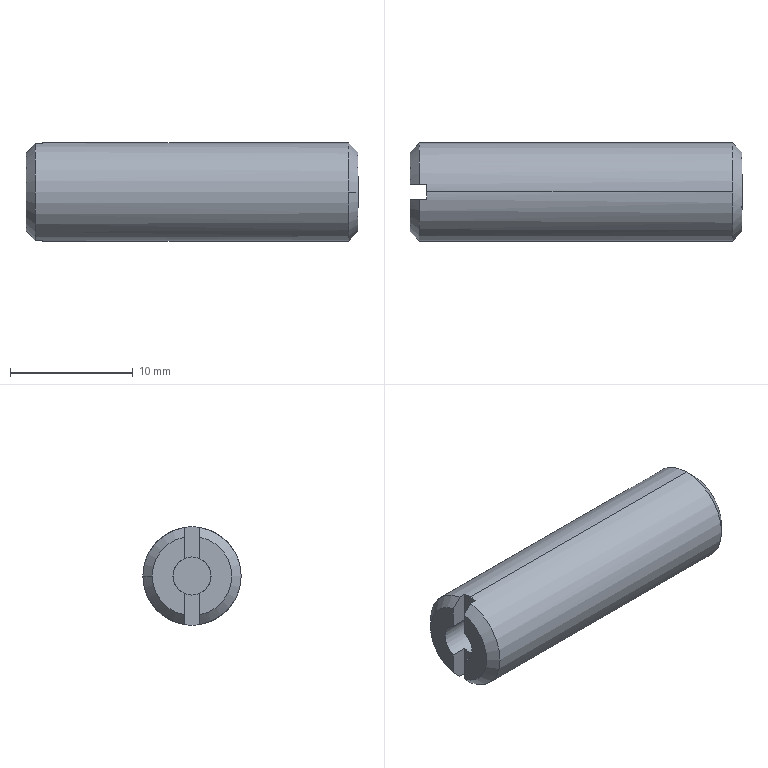Part | SolidWorks | features BaseBody 1 | 1 solid | 29 faces | box 27 x 8 x 8 mm | volume 931.32 mm3 | plane 18 | cylinder 6 | cone 5 | commonest cylinder face diameters 3.1 x2 4.8 x2 8 x2
STEP:
#1=CARTESIAN_POINT('',(26.233,4.,0.));
#2=VERTEX_POINT('',#1);
#3=CARTESIAN_POINT('',(26.233,0.,-4.));
#4=VERTEX_POINT('',#3);
#5=CARTESIAN_POINT('',(26.233,0.,0.));
#6=DIRECTION('',(-1.,0.,0.));
#7=DIRECTION('',(0.,0.,1.));
#8=AXIS2_PLACEMENT_3D('',#5,#6,#7);
#9=CIRCLE('',#8,4.);
#10=EDGE_CURVE('',#2,#4,#9,.T.);
#11=ORIENTED_EDGE('',*,*,#10,.T.);
#12=CARTESIAN_POINT('',(1.35,0.,-4.));
#13=VERTEX_POINT('',#12);
#14=CARTESIAN_POINT('',(27.,0.,-4.));
#15=DIRECTION('',(-1.,0.,0.));
#16=VECTOR('',#15,1000.);
#17=LINE('',#14,#16);
#18=EDGE_CURVE('',#4,#13,#17,.T.);
#19=ORIENTED_EDGE('',*,*,#18,.T.);
#20=CARTESIAN_POINT('',(1.35,0.62,-3.952));
#21=VERTEX_POINT('',#20);
#22=CARTESIAN_POINT('',(1.35,0.,0.));
#23=DIRECTION('',(1.,0.,0.));
#24=DIRECTION('',(0.,0.,1.));
#25=AXIS2_PLACEMENT_3D('',#22,#23,#24);
#26=CIRCLE('',#25,4.);
#27=EDGE_CURVE('',#13,#21,#26,.T.);
#28=ORIENTED_EDGE('',*,*,#27,.T.);
#29=CARTESIAN_POINT('',(0.767,0.62,-3.952));
#30=VERTEX_POINT('',#29);
#31=CARTESIAN_POINT('',(1.35,0.62,-3.952));
#32=DIRECTION('',(1.,0.,0.));
#33=VECTOR('',#32,1000.);
#34=LINE('',#31,#33);
#35=EDGE_CURVE('',#30,#21,#34,.T.);
#36=ORIENTED_EDGE('',*,*,#35,.F.);
#37=CARTESIAN_POINT('',(0.767,4.,0.));
#38=VERTEX_POINT('',#37);
#39=CARTESIAN_POINT('',(0.767,0.,0.));
#40=DIRECTION('',(1.,0.,0.));
#41=DIRECTION('',(0.,0.,1.));
#42=AXIS2_PLACEMENT_3D('',#39,#40,#41);
#43=CIRCLE('',#42,4.);
#44=EDGE_CURVE('',#30,#38,#43,.T.);
#45=ORIENTED_EDGE('',*,*,#44,.T.);
#46=CARTESIAN_POINT('',(0.767,0.62,3.952));
#47=VERTEX_POINT('',#46);
#48=CARTESIAN_POINT('',(0.767,0.,0.));
#49=DIRECTION('',(1.,0.,0.));
#50=DIRECTION('',(0.,0.,1.));
#51=AXIS2_PLACEMENT_3D('',#48,#49,#50);
#52=CIRCLE('',#51,4.);
#53=EDGE_CURVE('',#38,#47,#52,.T.);
#54=ORIENTED_EDGE('',*,*,#53,.T.);
#55=CARTESIAN_POINT('',(1.35,0.62,3.952));
#56=VERTEX_POINT('',#55);
#57=CARTESIAN_POINT('',(1.35,0.62,3.952));
#58=DIRECTION('',(-1.,0.,0.));
#59=VECTOR('',#58,1000.);
#60=LINE('',#57,#59);
#61=EDGE_CURVE('',#56,#47,#60,.T.);
#62=ORIENTED_EDGE('',*,*,#61,.F.);
#63=CARTESIAN_POINT('',(1.35,0.,4.));
#64=VERTEX_POINT('',#63);
#65=CARTESIAN_POINT('',(1.35,0.,0.));
#66=DIRECTION('',(1.,0.,0.));
#67=DIRECTION('',(0.,0.,1.));
#68=AXIS2_PLACEMENT_3D('',#65,#66,#67);
#69=CIRCLE('',#68,4.);
#70=EDGE_CURVE('',#56,#64,#69,.T.);
#71=ORIENTED_EDGE('',*,*,#70,.T.);
#72=CARTESIAN_POINT('',(26.233,0.,4.));
#73=VERTEX_POINT('',#72);
#74=CARTESIAN_POINT('',(27.,0.,4.));
#75=DIRECTION('',(-1.,0.,0.));
#76=VECTOR('',#75,1000.);
#77=LINE('',#74,#76);
#78=EDGE_CURVE('',#73,#64,#77,.T.);
#79=ORIENTED_EDGE('',*,*,#78,.F.);
#80=CARTESIAN_POINT('',(26.233,0.,0.));
#81=DIRECTION('',(-1.,0.,0.));
#82=DIRECTION('',(0.,0.,1.));
#83=AXIS2_PLACEMENT_3D('',#80,#81,#82);
#84=CIRCLE('',#83,4.);
#85=EDGE_CURVE('',#73,#2,#84,.T.);
#86=ORIENTED_EDGE('',*,*,#85,.T.);
#87=EDGE_LOOP('',(#11,#19,#28,#36,#45,#54,#62,#71,#79,#86));
#88=FACE_OUTER_BOUND('',#87,.T.);
#89=CARTESIAN_POINT('',(27.,0.,0.));
#90=DIRECTION('',(-1.,0.,0.));
#91=DIRECTION('',(0.,0.,1.));
#92=AXIS2_PLACEMENT_3D('',#89,#90,#91);
#93=CYLINDRICAL_SURFACE('',#92,4.);
#94=ADVANCED_FACE('',(#88),#93,.T.);
#95=CARTESIAN_POINT('',(27.,-3.233,0.));
#96=VERTEX_POINT('',#95);
#97=CARTESIAN_POINT('',(27.,3.233,0.));
#98=VERTEX_POINT('',#97);
#99=CARTESIAN_POINT('',(27.,0.,0.));
#100=DIRECTION('',(-1.,0.,0.));
#101=DIRECTION('',(0.,-1.,0.));
#102=AXIS2_PLACEMENT_3D('',#99,#100,#101);
#103=CIRCLE('',#102,3.233);
#104=EDGE_CURVE('',#96,#98,#103,.T.);
#105=ORIENTED_EDGE('',*,*,#104,.T.);
#106=CARTESIAN_POINT('',(26.233,4.,0.));
#107=DIRECTION('',(-0.7071,0.7071,0.));
#108=VECTOR('',#107,1000.);
#109=LINE('',#106,#108);
#110=EDGE_CURVE('',#98,#2,#109,.T.);
#111=ORIENTED_EDGE('',*,*,#110,.T.);
#112=ORIENTED_EDGE('',*,*,#85,.F.);
#113=CARTESIAN_POINT('',(26.233,-4.,0.));
#114=VERTEX_POINT('',#113);
#115=CARTESIAN_POINT('',(26.233,0.,0.));
#116=DIRECTION('',(-1.,0.,0.));
#117=DIRECTION('',(0.,0.,1.));
#118=AXIS2_PLACEMENT_3D('',#115,#116,#117);
#119=CIRCLE('',#118,4.);
#120=EDGE_CURVE('',#114,#73,#119,.T.);
#121=ORIENTED_EDGE('',*,*,#120,.F.);
#122=CARTESIAN_POINT('',(26.233,-4.,0.));
#123=DIRECTION('',(-0.7071,-0.7071,0.));
#124=VECTOR('',#123,1000.);
#125=LINE('',#122,#124);
#126=EDGE_CURVE('',#96,#114,#125,.T.);
#127=ORIENTED_EDGE('',*,*,#126,.F.);
#128=EDGE_LOOP('',(#105,#111,#112,#121,#127));
#129=FACE_OUTER_BOUND('',#128,.T.);
#130=CARTESIAN_POINT('',(26.233,0.,0.));
#131=DIRECTION('',(-1.,0.,0.));
#132=DIRECTION('',(0.,-1.,0.));
#133=AXIS2_PLACEMENT_3D('',#130,#131,#132);
#134=CONICAL_SURFACE('',#133,4.,0.7854);
#135=ADVANCED_FACE('',(#129),#134,.T.);
#136=CARTESIAN_POINT('',(0.,0.62,-3.173));
#137=VERTEX_POINT('',#136);
#138=CARTESIAN_POINT('',(0.,3.233,0.));
#139=VERTEX_POINT('',#138);
#140=CARTESIAN_POINT('',(0.,0.,0.));
#141=DIRECTION('',(1.,0.,0.));
#142=DIRECTION('',(0.,1.,0.));
#143=AXIS2_PLACEMENT_3D('',#140,#141,#142);
#144=CIRCLE('',#143,3.233);
#145=EDGE_CURVE('',#137,#139,#144,.T.);
#146=ORIENTED_EDGE('',*,*,#145,.T.);
#147=CARTESIAN_POINT('',(0.767,4.,0.));
#148=DIRECTION('',(0.7071,0.7071,0.));
#149=VECTOR('',#148,1000.);
#150=LINE('',#147,#149);
#151=EDGE_CURVE('',#139,#38,#150,.T.);
#152=ORIENTED_EDGE('',*,*,#151,.T.);
#153=ORIENTED_EDGE('',*,*,#44,.F.);
#154=CARTESIAN_POINT('',(0.,0.62,-3.173));
#155=CARTESIAN_POINT('',(0.2552,0.62,-3.433));
#156=CARTESIAN_POINT('',(0.511,0.62,-3.692));
#157=CARTESIAN_POINT('',(0.767,0.62,-3.952));
#158=B_SPLINE_CURVE_WITH_KNOTS('',3,(#154,#155,#156,#157),.UNSPECIFIED.,.F.,.F.,(4,4),(0.,0.001093),.UNSPECIFIED.);
#159=EDGE_CURVE('',#137,#30,#158,.T.);
#160=ORIENTED_EDGE('',*,*,#159,.F.);
#161=EDGE_LOOP('',(#146,#152,#153,#160));
#162=FACE_OUTER_BOUND('',#161,.T.);
#163=CARTESIAN_POINT('',(0.767,0.,0.));
#164=DIRECTION('',(1.,0.,0.));
#165=DIRECTION('',(0.,1.,0.));
#166=AXIS2_PLACEMENT_3D('',#163,#164,#165);
#167=CONICAL_SURFACE('',#166,4.,0.7854);
#168=ADVANCED_FACE('',(#162),#167,.T.);
#169=CARTESIAN_POINT('',(4.5,0.,-1.55));
#170=VERTEX_POINT('',#169);
#171=CARTESIAN_POINT('',(4.5,0.,1.55));
#172=VERTEX_POINT('',#171);
#173=CARTESIAN_POINT('',(4.5,0.,0.));
#174=DIRECTION('',(-1.,0.,0.));
#175=DIRECTION('',(0.,0.,1.));
#176=AXIS2_PLACEMENT_3D('',#173,#174,#175);
#177=CIRCLE('',#176,1.55);
#178=EDGE_CURVE('',#170,#172,#177,.T.);
#179=ORIENTED_EDGE('',*,*,#178,.F.);
#180=CARTESIAN_POINT('',(1.35,0.,-1.55));
#181=VERTEX_POINT('',#180);
#182=CARTESIAN_POINT('',(27.,0.,-1.55));
#183=DIRECTION('',(-1.,0.,0.));
#184=VECTOR('',#183,1000.);
#185=LINE('',#182,#184);
#186=EDGE_CURVE('',#170,#181,#185,.T.);
#187=ORIENTED_EDGE('',*,*,#186,.T.);
#188=CARTESIAN_POINT('',(1.35,-0.62,-1.421));
#189=VERTEX_POINT('',#188);
#190=CARTESIAN_POINT('',(1.35,0.,0.));
#191=DIRECTION('',(1.,0.,0.));
#192=DIRECTION('',(0.,0.,1.));
#193=AXIS2_PLACEMENT_3D('',#190,#191,#192);
#194=CIRCLE('',#193,1.55);
#195=EDGE_CURVE('',#189,#181,#194,.T.);
#196=ORIENTED_EDGE('',*,*,#195,.F.);
#197=CARTESIAN_POINT('',(0.,-0.62,-1.421));
#198=VERTEX_POINT('',#197);
#199=CARTESIAN_POINT('',(27.,-0.62,-1.421));
#200=DIRECTION('',(1.,0.,0.));
#201=VECTOR('',#200,1000.);
#202=LINE('',#199,#201);
#203=EDGE_CURVE('',#198,#189,#202,.T.);
#204=ORIENTED_EDGE('',*,*,#203,.F.);
#205=CARTESIAN_POINT('',(0.,-0.62,1.421));
#206=VERTEX_POINT('',#205);
#207=CARTESIAN_POINT('',(0.,0.,0.));
#208=DIRECTION('',(-1.,0.,0.));
#209=DIRECTION('',(0.,0.,1.));
#210=AXIS2_PLACEMENT_3D('',#207,#208,#209);
#211=CIRCLE('',#210,1.55);
#212=EDGE_CURVE('',#198,#206,#211,.T.);
#213=ORIENTED_EDGE('',*,*,#212,.T.);
#214=CARTESIAN_POINT('',(1.35,-0.62,1.421));
#215=VERTEX_POINT('',#214);
#216=CARTESIAN_POINT('',(1.35,-0.62,1.421));
#217=DIRECTION('',(-1.,0.,0.));
#218=VECTOR('',#217,1000.);
#219=LINE('',#216,#218);
#220=EDGE_CURVE('',#215,#206,#219,.T.);
#221=ORIENTED_EDGE('',*,*,#220,.F.);
#222=CARTESIAN_POINT('',(1.35,0.,1.55));
#223=VERTEX_POINT('',#222);
#224=CARTESIAN_POINT('',(1.35,0.,0.));
#225=DIRECTION('',(1.,0.,0.));
#226=DIRECTION('',(0.,0.,1.));
#227=AXIS2_PLACEMENT_3D('',#224,#225,#226);
#228=CIRCLE('',#227,1.55);
#229=EDGE_CURVE('',#223,#215,#228,.T.);
#230=ORIENTED_EDGE('',*,*,#229,.F.);
#231=CARTESIAN_POINT('',(27.,0.,1.55));
#232=DIRECTION('',(-1.,0.,0.));
#233=VECTOR('',#232,1000.);
#234=LINE('',#231,#233);
#235=EDGE_CURVE('',#172,#223,#234,.T.);
#236=ORIENTED_EDGE('',*,*,#235,.F.);
#237=EDGE_LOOP('',(#179,#187,#196,#204,#213,#221,#230,#236));
#238=FACE_OUTER_BOUND('',#237,.T.);
#239=CARTESIAN_POINT('',(27.,0.,0.));
#240=DIRECTION('',(-1.,0.,0.));
#241=DIRECTION('',(0.,0.,1.));
#242=AXIS2_PLACEMENT_3D('',#239,#240,#241);
#243=CYLINDRICAL_SURFACE('',#242,1.55);
#244=ADVANCED_FACE('',(#238),#243,.F.);
#245=CARTESIAN_POINT('',(24.57,0.,-2.4));
#246=VERTEX_POINT('',#245);
#247=CARTESIAN_POINT('',(24.57,0.,2.4));
#248=VERTEX_POINT('',#247);
#249=CARTESIAN_POINT('',(24.57,0.,0.));
#250=DIRECTION('',(-1.,0.,0.));
#251=DIRECTION('',(0.,0.,1.));
#252=AXIS2_PLACEMENT_3D('',#249,#250,#251);
#253=CIRCLE('',#252,2.4);
#254=EDGE_CURVE('',#246,#248,#253,.T.);
#255=ORIENTED_EDGE('',*,*,#254,.F.);
#256=CARTESIAN_POINT('',(4.5,0.,-2.4));
#257=VERTEX_POINT('',#256);
#258=CARTESIAN_POINT('',(27.,0.,-2.4));
#259=DIRECTION('',(-1.,0.,0.));
#260=VECTOR('',#259,1000.);
#261=LINE('',#258,#260);
#262=EDGE_CURVE('',#246,#257,#261,.T.);
#263=ORIENTED_EDGE('',*,*,#262,.T.);
#264=CARTESIAN_POINT('',(4.5,0.,2.4));
#265=VERTEX_POINT('',#264);
#266=CARTESIAN_POINT('',(4.5,0.,0.));
#267=DIRECTION('',(-1.,0.,0.));
#268=DIRECTION('',(0.,0.,1.));
#269=AXIS2_PLACEMENT_3D('',#266,#267,#268);
#270=CIRCLE('',#269,2.4);
#271=EDGE_CURVE('',#257,#265,#270,.T.);
#272=ORIENTED_EDGE('',*,*,#271,.T.);
#273=CARTESIAN_POINT('',(27.,0.,2.4));
#274=DIRECTION('',(-1.,0.,0.));
#275=VECTOR('',#274,1000.);
#276=LINE('',#273,#275);
#277=EDGE_CURVE('',#248,#265,#276,.T.);
#278=ORIENTED_EDGE('',*,*,#277,.F.);
#279=EDGE_LOOP('',(#255,#263,#272,#278));
#280=FACE_OUTER_BOUND('',#279,.T.);
#281=CARTESIAN_POINT('',(27.,0.,0.));
#282=DIRECTION('',(-1.,0.,0.));
#283=DIRECTION('',(0.,0.,1.));
#284=AXIS2_PLACEMENT_3D('',#281,#282,#283);
#285=CYLINDRICAL_SURFACE('',#284,2.4);
#286=ADVANCED_FACE('',(#280),#285,.F.);
#287=ORIENTED_EDGE('',*,*,#18,.F.);
#288=CARTESIAN_POINT('',(26.233,0.,0.));
#289=DIRECTION('',(-1.,0.,0.));
#290=DIRECTION('',(0.,0.,1.));
#291=AXIS2_PLACEMENT_3D('',#288,#289,#290);
#292=CIRCLE('',#291,4.);
#293=EDGE_CURVE('',#4,#114,#292,.T.);
#294=ORIENTED_EDGE('',*,*,#293,.T.);
#295=ORIENTED_EDGE('',*,*,#120,.T.);
#296=ORIENTED_EDGE('',*,*,#78,.T.);
#297=CARTESIAN_POINT('',(1.35,-0.62,3.952));
#298=VERTEX_POINT('',#297);
#299=CARTESIAN_POINT('',(1.35,0.,0.));
#300=DIRECTION('',(1.,0.,0.));
#301=DIRECTION('',(0.,0.,1.));
#302=AXIS2_PLACEMENT_3D('',#299,#300,#301);
#303=CIRCLE('',#302,4.);
#304=EDGE_CURVE('',#64,#298,#303,.T.);
#305=ORIENTED_EDGE('',*,*,#304,.T.);
#306=CARTESIAN_POINT('',(0.767,-0.62,3.952));
#307=VERTEX_POINT('',#306);
#308=CARTESIAN_POINT('',(1.35,-0.62,3.952));
#309=DIRECTION('',(1.,0.,0.));
#310=VECTOR('',#309,1000.);
#311=LINE('',#308,#310);
#312=EDGE_CURVE('',#307,#298,#311,.T.);
#313=ORIENTED_EDGE('',*,*,#312,.F.);
#314=CARTESIAN_POINT('',(0.767,-0.62,-3.952));
#315=VERTEX_POINT('',#314);
#316=CARTESIAN_POINT('',(0.767,0.,0.));
#317=DIRECTION('',(1.,0.,0.));
#318=DIRECTION('',(0.,0.,1.));
#319=AXIS2_PLACEMENT_3D('',#316,#317,#318);
#320=CIRCLE('',#319,4.);
#321=EDGE_CURVE('',#307,#315,#320,.T.);
#322=ORIENTED_EDGE('',*,*,#321,.T.);
#323=CARTESIAN_POINT('',(1.35,-0.62,-3.952));
#324=VERTEX_POINT('',#323);
#325=CARTESIAN_POINT('',(1.35,-0.62,-3.952));
#326=DIRECTION('',(-1.,0.,0.));
#327=VECTOR('',#326,1000.);
#328=LINE('',#325,#327);
#329=EDGE_CURVE('',#324,#315,#328,.T.);
#330=ORIENTED_EDGE('',*,*,#329,.F.);
#331=CARTESIAN_POINT('',(1.35,0.,0.));
#332=DIRECTION('',(1.,0.,0.));
#333=DIRECTION('',(0.,0.,1.));
#334=AXIS2_PLACEMENT_3D('',#331,#332,#333);
#335=CIRCLE('',#334,4.);
#336=EDGE_CURVE('',#324,#13,#335,.T.);
#337=ORIENTED_EDGE('',*,*,#336,.T.);
#338=EDGE_LOOP('',(#287,#294,#295,#296,#305,#313,#322,#330,#337));
#339=FACE_OUTER_BOUND('',#338,.T.);
#340=CARTESIAN_POINT('',(27.,0.,0.));
#341=DIRECTION('',(-1.,0.,0.));
#342=DIRECTION('',(0.,0.,1.));
#343=AXIS2_PLACEMENT_3D('',#340,#341,#342);
#344=CYLINDRICAL_SURFACE('',#343,4.);
#345=ADVANCED_FACE('',(#339),#344,.T.);
#346=CARTESIAN_POINT('',(0.,-0.62,-3.173));
#347=VERTEX_POINT('',#346);
#348=CARTESIAN_POINT('',(0.767,-0.62,-3.952));
#349=CARTESIAN_POINT('',(0.511,-0.62,-3.692));
#350=CARTESIAN_POINT('',(0.2552,-0.62,-3.433));
#351=CARTESIAN_POINT('',(0.,-0.62,-3.173));
#352=B_SPLINE_CURVE_WITH_KNOTS('',3,(#348,#349,#350,#351),.UNSPECIFIED.,.F.,.F.,(4,4),(0.,0.001093),.UNSPECIFIED.);
#353=EDGE_CURVE('',#315,#347,#352,.T.);
#354=ORIENTED_EDGE('',*,*,#353,.F.);
#355=ORIENTED_EDGE('',*,*,#321,.F.);
#356=CARTESIAN_POINT('',(0.,-0.62,3.173));
#357=VERTEX_POINT('',#356);
#358=CARTESIAN_POINT('',(0.,-0.62,3.173));
#359=CARTESIAN_POINT('',(0.2552,-0.62,3.433));
#360=CARTESIAN_POINT('',(0.511,-0.62,3.692));
#361=CARTESIAN_POINT('',(0.767,-0.62,3.952));
#362=B_SPLINE_CURVE_WITH_KNOTS('',3,(#358,#359,#360,#361),.UNSPECIFIED.,.F.,.F.,(4,4),(0.,0.001093),.UNSPECIFIED.);
#363=EDGE_CURVE('',#357,#307,#362,.T.);
#364=ORIENTED_EDGE('',*,*,#363,.F.);
#365=CARTESIAN_POINT('',(0.,0.,0.));
#366=DIRECTION('',(1.,0.,0.));
#367=DIRECTION('',(0.,1.,0.));
#368=AXIS2_PLACEMENT_3D('',#365,#366,#367);
#369=CIRCLE('',#368,3.233);
#370=EDGE_CURVE('',#357,#347,#369,.T.);
#371=ORIENTED_EDGE('',*,*,#370,.T.);
#372=EDGE_LOOP('',(#354,#355,#364,#371));
#373=FACE_OUTER_BOUND('',#372,.T.);
#374=CARTESIAN_POINT('',(0.767,0.,0.));
#375=DIRECTION('',(1.,0.,0.));
#376=DIRECTION('',(0.,1.,0.));
#377=AXIS2_PLACEMENT_3D('',#374,#375,#376);
#378=CONICAL_SURFACE('',#377,4.,0.7854);
#379=ADVANCED_FACE('',(#373),#378,.T.);
#380=ORIENTED_EDGE('',*,*,#110,.F.);
#381=CARTESIAN_POINT('',(27.,0.,0.));
#382=DIRECTION('',(-1.,0.,0.));
#383=DIRECTION('',(0.,-1.,0.));
#384=AXIS2_PLACEMENT_3D('',#381,#382,#383);
#385=CIRCLE('',#384,3.233);
#386=EDGE_CURVE('',#98,#96,#385,.T.);
#387=ORIENTED_EDGE('',*,*,#386,.T.);
#388=ORIENTED_EDGE('',*,*,#126,.T.);
#389=ORIENTED_EDGE('',*,*,#293,.F.);
#390=ORIENTED_EDGE('',*,*,#10,.F.);
#391=EDGE_LOOP('',(#380,#387,#388,#389,#390));
#392=FACE_OUTER_BOUND('',#391,.T.);
#393=CARTESIAN_POINT('',(26.233,0.,0.));
#394=DIRECTION('',(-1.,0.,0.));
#395=DIRECTION('',(0.,-1.,0.));
#396=AXIS2_PLACEMENT_3D('',#393,#394,#395);
#397=CONICAL_SURFACE('',#396,4.,0.7854);
#398=ADVANCED_FACE('',(#392),#397,.T.);
#399=CARTESIAN_POINT('',(0.,-0.62,0.));
#400=DIRECTION('',(0.,0.,1.));
#401=VECTOR('',#400,1000.);
#402=LINE('',#399,#401);
#403=EDGE_CURVE('',#206,#357,#402,.T.);
#404=ORIENTED_EDGE('',*,*,#403,.F.);
#405=ORIENTED_EDGE('',*,*,#212,.F.);
#406=CARTESIAN_POINT('',(0.,-0.62,0.));
#407=DIRECTION('',(0.,0.,1.));
#408=VECTOR('',#407,1000.);
#409=LINE('',#406,#408);
#410=EDGE_CURVE('',#347,#198,#409,.T.);
#411=ORIENTED_EDGE('',*,*,#410,.F.);
#412=ORIENTED_EDGE('',*,*,#370,.F.);
#413=EDGE_LOOP('',(#404,#405,#411,#412));
#414=FACE_OUTER_BOUND('',#413,.T.);
#415=CARTESIAN_POINT('',(0.,1.55,0.));
#416=DIRECTION('',(1.,0.,0.));
#417=DIRECTION('',(0.,0.,-1.));
#418=AXIS2_PLACEMENT_3D('',#415,#416,#417);
#419=PLANE('',#418);
#420=ADVANCED_FACE('',(#414),#419,.F.);
#421=ORIENTED_EDGE('',*,*,#151,.F.);
#422=CARTESIAN_POINT('',(0.,0.62,3.173));
#423=VERTEX_POINT('',#422);
#424=CARTESIAN_POINT('',(0.,0.,0.));
#425=DIRECTION('',(1.,0.,0.));
#426=DIRECTION('',(0.,1.,0.));
#427=AXIS2_PLACEMENT_3D('',#424,#425,#426);
#428=CIRCLE('',#427,3.233);
#429=EDGE_CURVE('',#139,#423,#428,.T.);
#430=ORIENTED_EDGE('',*,*,#429,.T.);
#431=CARTESIAN_POINT('',(0.767,0.62,3.952));
#432=CARTESIAN_POINT('',(0.511,0.62,3.692));
#433=CARTESIAN_POINT('',(0.2552,0.62,3.433));
#434=CARTESIAN_POINT('',(0.,0.62,3.173));
#435=B_SPLINE_CURVE_WITH_KNOTS('',3,(#431,#432,#433,#434),.UNSPECIFIED.,.F.,.F.,(4,4),(0.,0.001093),.UNSPECIFIED.);
#436=EDGE_CURVE('',#47,#423,#435,.T.);
#437=ORIENTED_EDGE('',*,*,#436,.F.);
#438=ORIENTED_EDGE('',*,*,#53,.F.);
#439=EDGE_LOOP('',(#421,#430,#437,#438));
#440=FACE_OUTER_BOUND('',#439,.T.);
#441=CARTESIAN_POINT('',(0.767,0.,0.));
#442=DIRECTION('',(1.,0.,0.));
#443=DIRECTION('',(0.,1.,0.));
#444=AXIS2_PLACEMENT_3D('',#441,#442,#443);
#445=CONICAL_SURFACE('',#444,4.,0.7854);
#446=ADVANCED_FACE('',(#440),#445,.T.);
#447=CARTESIAN_POINT('',(27.,-0.7217,-1.25));
#448=VERTEX_POINT('',#447);
#449=CARTESIAN_POINT('',(27.,0.7217,-1.25));
#450=VERTEX_POINT('',#449);
#451=CARTESIAN_POINT('',(27.,3.233,-1.25));
#452=DIRECTION('',(0.,1.,0.));
#453=VECTOR('',#452,1000.);
#454=LINE('',#451,#453);
#455=EDGE_CURVE('',#448,#450,#454,.T.);
#456=ORIENTED_EDGE('',*,*,#455,.F.);
#457=CARTESIAN_POINT('',(27.,-1.443,0.));
#458=VERTEX_POINT('',#457);
#459=CARTESIAN_POINT('',(27.,-1.443,0.));
#460=DIRECTION('',(0.,0.5,-0.866));
#461=VECTOR('',#460,1000.);
#462=LINE('',#459,#461);
#463=EDGE_CURVE('',#458,#448,#462,.T.);
#464=ORIENTED_EDGE('',*,*,#463,.F.);
#465=CARTESIAN_POINT('',(27.,-0.7217,1.25));
#466=VERTEX_POINT('',#465);
#467=CARTESIAN_POINT('',(27.,-0.7217,1.25));
#468=DIRECTION('',(0.,-0.5,-0.866));
#469=VECTOR('',#468,1000.);
#470=LINE('',#467,#469);
#471=EDGE_CURVE('',#466,#458,#470,.T.);
#472=ORIENTED_EDGE('',*,*,#471,.F.);
#473=CARTESIAN_POINT('',(27.,0.7217,1.25));
#474=VERTEX_POINT('',#473);
#475=CARTESIAN_POINT('',(27.,3.233,1.25));
#476=DIRECTION('',(0.,-1.,0.));
#477=VECTOR('',#476,1000.);
#478=LINE('',#475,#477);
#479=EDGE_CURVE('',#474,#466,#478,.T.);
#480=ORIENTED_EDGE('',*,*,#479,.F.);
#481=CARTESIAN_POINT('',(27.,1.443,0.));
#482=VERTEX_POINT('',#481);
#483=CARTESIAN_POINT('',(27.,1.443,0.));
#484=DIRECTION('',(0.,-0.5,0.866));
#485=VECTOR('',#484,1000.);
#486=LINE('',#483,#485);
#487=EDGE_CURVE('',#482,#474,#486,.T.);
#488=ORIENTED_EDGE('',*,*,#487,.F.);
#489=CARTESIAN_POINT('',(27.,0.7217,-1.25));
#490=DIRECTION('',(0.,0.5,0.866));
#491=VECTOR('',#490,1000.);
#492=LINE('',#489,#491);
#493=EDGE_CURVE('',#450,#482,#492,.T.);
#494=ORIENTED_EDGE('',*,*,#493,.F.);
#495=EDGE_LOOP('',(#456,#464,#472,#480,#488,#494));
#496=FACE_BOUND('',#495,.T.);
#497=ORIENTED_EDGE('',*,*,#104,.F.);
#498=ORIENTED_EDGE('',*,*,#386,.F.);
#499=EDGE_LOOP('',(#497,#498));
#500=FACE_OUTER_BOUND('',#499,.T.);
#501=CARTESIAN_POINT('',(27.,3.233,0.));
#502=DIRECTION('',(-1.,0.,0.));
#503=DIRECTION('',(0.,0.,1.));
#504=AXIS2_PLACEMENT_3D('',#501,#502,#503);
#505=PLANE('',#504);
#506=ADVANCED_FACE('',(#496,#500),#505,.F.);
#507=ORIENTED_EDGE('',*,*,#403,.T.);
#508=ORIENTED_EDGE('',*,*,#363,.T.);
#509=ORIENTED_EDGE('',*,*,#312,.T.);
#510=CARTESIAN_POINT('',(1.35,-0.62,8.));
#511=DIRECTION('',(0.,0.,-1.));
#512=VECTOR('',#511,1000.);
#513=LINE('',#510,#512);
#514=EDGE_CURVE('',#298,#215,#513,.T.);
#515=ORIENTED_EDGE('',*,*,#514,.T.);
#516=ORIENTED_EDGE('',*,*,#220,.T.);
#517=EDGE_LOOP('',(#507,#508,#509,#515,#516));
#518=FACE_OUTER_BOUND('',#517,.T.);
#519=CARTESIAN_POINT('',(1.35,-0.62,8.));
#520=DIRECTION('',(0.,1.,0.));
#521=DIRECTION('',(0.,0.,1.));
#522=AXIS2_PLACEMENT_3D('',#519,#520,#521);
#523=PLANE('',#522);
#524=ADVANCED_FACE('',(#518),#523,.T.);
#525=ORIENTED_EDGE('',*,*,#186,.F.);
#526=CARTESIAN_POINT('',(4.5,0.,0.));
#527=DIRECTION('',(-1.,0.,0.));
#528=DIRECTION('',(0.,0.,1.));
#529=AXIS2_PLACEMENT_3D('',#526,#527,#528);
#530=CIRCLE('',#529,1.55);
#531=EDGE_CURVE('',#172,#170,#530,.T.);
#532=ORIENTED_EDGE('',*,*,#531,.F.);
#533=ORIENTED_EDGE('',*,*,#235,.T.);
#534=CARTESIAN_POINT('',(1.35,0.62,1.421));
#535=VERTEX_POINT('',#534);
#536=CARTESIAN_POINT('',(1.35,0.,0.));
#537=DIRECTION('',(1.,0.,0.));
#538=DIRECTION('',(0.,0.,1.));
#539=AXIS2_PLACEMENT_3D('',#536,#537,#538);
#540=CIRCLE('',#539,1.55);
#541=EDGE_CURVE('',#535,#223,#540,.T.);
#542=ORIENTED_EDGE('',*,*,#541,.F.);
#543=CARTESIAN_POINT('',(0.,0.62,1.421));
#544=VERTEX_POINT('',#543);
#545=CARTESIAN_POINT('',(27.,0.62,1.421));
#546=DIRECTION('',(1.,0.,0.));
#547=VECTOR('',#546,1000.);
#548=LINE('',#545,#547);
#549=EDGE_CURVE('',#544,#535,#548,.T.);
#550=ORIENTED_EDGE('',*,*,#549,.F.);
#551=CARTESIAN_POINT('',(0.,0.62,-1.421));
#552=VERTEX_POINT('',#551);
#553=CARTESIAN_POINT('',(0.,0.,0.));
#554=DIRECTION('',(-1.,0.,0.));
#555=DIRECTION('',(0.,0.,1.));
#556=AXIS2_PLACEMENT_3D('',#553,#554,#555);
#557=CIRCLE('',#556,1.55);
#558=EDGE_CURVE('',#544,#552,#557,.T.);
#559=ORIENTED_EDGE('',*,*,#558,.T.);
#560=CARTESIAN_POINT('',(1.35,0.62,-1.421));
#561=VERTEX_POINT('',#560);
#562=CARTESIAN_POINT('',(27.,0.62,-1.421));
#563=DIRECTION('',(-1.,0.,0.));
#564=VECTOR('',#563,1000.);
#565=LINE('',#562,#564);
#566=EDGE_CURVE('',#561,#552,#565,.T.);
#567=ORIENTED_EDGE('',*,*,#566,.F.);
#568=CARTESIAN_POINT('',(1.35,0.,0.));
#569=DIRECTION('',(1.,0.,0.));
#570=DIRECTION('',(0.,0.,1.));
#571=AXIS2_PLACEMENT_3D('',#568,#569,#570);
#572=CIRCLE('',#571,1.55);
#573=EDGE_CURVE('',#181,#561,#572,.T.);
#574=ORIENTED_EDGE('',*,*,#573,.F.);
#575=EDGE_LOOP('',(#525,#532,#533,#542,#550,#559,#567,#574));
#576=FACE_OUTER_BOUND('',#575,.T.);
#577=CARTESIAN_POINT('',(27.,0.,0.));
#578=DIRECTION('',(-1.,0.,0.));
#579=DIRECTION('',(0.,0.,1.));
#580=AXIS2_PLACEMENT_3D('',#577,#578,#579);
#581=CYLINDRICAL_SURFACE('',#580,1.55);
#582=ADVANCED_FACE('',(#576),#581,.F.);
#583=CARTESIAN_POINT('',(1.35,-0.62,8.));
#584=DIRECTION('',(0.,0.,-1.));
#585=VECTOR('',#584,1000.);
#586=LINE('',#583,#585);
#587=EDGE_CURVE('',#189,#324,#586,.T.);
#588=ORIENTED_EDGE('',*,*,#587,.T.);
#589=ORIENTED_EDGE('',*,*,#329,.T.);
#590=ORIENTED_EDGE('',*,*,#353,.T.);
#591=ORIENTED_EDGE('',*,*,#410,.T.);
#592=ORIENTED_EDGE('',*,*,#203,.T.);
#593=EDGE_LOOP('',(#588,#589,#590,#591,#592));
#594=FACE_OUTER_BOUND('',#593,.T.);
#595=CARTESIAN_POINT('',(1.35,-0.62,8.));
#596=DIRECTION('',(0.,1.,0.));
#597=DIRECTION('',(0.,0.,1.));
#598=AXIS2_PLACEMENT_3D('',#595,#596,#597);
#599=PLANE('',#598);
#600=ADVANCED_FACE('',(#594),#599,.T.);
#601=CARTESIAN_POINT('',(0.,0.62,0.));
#602=DIRECTION('',(0.,0.,-1.));
#603=VECTOR('',#602,1000.);
#604=LINE('',#601,#603);
#605=EDGE_CURVE('',#423,#544,#604,.T.);
#606=ORIENTED_EDGE('',*,*,#605,.F.);
#607=ORIENTED_EDGE('',*,*,#429,.F.);
#608=ORIENTED_EDGE('',*,*,#145,.F.);
#609=CARTESIAN_POINT('',(0.,0.62,0.));
#610=DIRECTION('',(0.,0.,-1.));
#611=VECTOR('',#610,1000.);
#612=LINE('',#609,#611);
#613=EDGE_CURVE('',#552,#137,#612,.T.);
#614=ORIENTED_EDGE('',*,*,#613,.F.);
#615=ORIENTED_EDGE('',*,*,#558,.F.);
#616=EDGE_LOOP('',(#606,#607,#608,#614,#615));
#617=FACE_OUTER_BOUND('',#616,.T.);
#618=CARTESIAN_POINT('',(0.,1.55,0.));
#619=DIRECTION('',(1.,0.,0.));
#620=DIRECTION('',(0.,0.,-1.));
#621=AXIS2_PLACEMENT_3D('',#618,#619,#620);
#622=PLANE('',#621);
#623=ADVANCED_FACE('',(#617),#622,.F.);
#624=CARTESIAN_POINT('',(25.65,0.7217,-1.25));
#625=VERTEX_POINT('',#624);
#626=CARTESIAN_POINT('',(25.65,1.443,0.));
#627=VERTEX_POINT('',#626);
#628=CARTESIAN_POINT('',(25.65,0.7217,-1.25));
#629=DIRECTION('',(0.,0.5,0.866));
#630=VECTOR('',#629,1000.);
#631=LINE('',#628,#630);
#632=EDGE_CURVE('',#625,#627,#631,.T.);
#633=ORIENTED_EDGE('',*,*,#632,.F.);
#634=CARTESIAN_POINT('',(25.65,0.7217,-1.25));
#635=DIRECTION('',(-1.,0.,0.));
#636=VECTOR('',#635,1000.);
#637=LINE('',#634,#636);
#638=EDGE_CURVE('',#450,#625,#637,.T.);
#639=ORIENTED_EDGE('',*,*,#638,.F.);
#640=ORIENTED_EDGE('',*,*,#493,.T.);
#641=CARTESIAN_POINT('',(25.65,1.443,0.));
#642=DIRECTION('',(1.,0.,0.));
#643=VECTOR('',#642,1000.);
#644=LINE('',#641,#643);
#645=EDGE_CURVE('',#627,#482,#644,.T.);
#646=ORIENTED_EDGE('',*,*,#645,.F.);
#647=EDGE_LOOP('',(#633,#639,#640,#646));
#648=FACE_OUTER_BOUND('',#647,.T.);
#649=CARTESIAN_POINT('',(25.65,0.7217,-1.25));
#650=DIRECTION('',(0.,0.866,-0.5));
#651=DIRECTION('',(0.,0.5,0.866));
#652=AXIS2_PLACEMENT_3D('',#649,#650,#651);
#653=PLANE('',#652);
#654=ADVANCED_FACE('',(#648),#653,.F.);
#655=CARTESIAN_POINT('',(25.65,-0.7217,-1.25));
#656=VERTEX_POINT('',#655);
#657=CARTESIAN_POINT('',(25.65,-0.7217,-1.25));
#658=DIRECTION('',(0.,1.,0.));
#659=VECTOR('',#658,1000.);
#660=LINE('',#657,#659);
#661=EDGE_CURVE('',#656,#625,#660,.T.);
#662=ORIENTED_EDGE('',*,*,#661,.F.);
#663=CARTESIAN_POINT('',(25.65,-0.7217,-1.25));
#664=DIRECTION('',(-1.,0.,0.));
#665=VECTOR('',#664,1000.);
#666=LINE('',#663,#665);
#667=EDGE_CURVE('',#448,#656,#666,.T.);
#668=ORIENTED_EDGE('',*,*,#667,.F.);
#669=ORIENTED_EDGE('',*,*,#455,.T.);
#670=ORIENTED_EDGE('',*,*,#638,.T.);
#671=EDGE_LOOP('',(#662,#668,#669,#670));
#672=FACE_OUTER_BOUND('',#671,.T.);
#673=CARTESIAN_POINT('',(25.65,-0.7217,-1.25));
#674=DIRECTION('',(0.,0.,-1.));
#675=DIRECTION('',(-1.,0.,0.));
#676=AXIS2_PLACEMENT_3D('',#673,#674,#675);
#677=PLANE('',#676);
#678=ADVANCED_FACE('',(#672),#677,.F.);
#679=CARTESIAN_POINT('',(25.65,-1.443,0.));
#680=VERTEX_POINT('',#679);
#681=CARTESIAN_POINT('',(25.65,-1.443,0.));
#682=DIRECTION('',(0.,0.5,-0.866));
#683=VECTOR('',#682,1000.);
#684=LINE('',#681,#683);
#685=EDGE_CURVE('',#680,#656,#684,.T.);
#686=ORIENTED_EDGE('',*,*,#685,.F.);
#687=CARTESIAN_POINT('',(25.65,-1.443,0.));
#688=DIRECTION('',(-1.,0.,0.));
#689=VECTOR('',#688,1000.);
#690=LINE('',#687,#689);
#691=EDGE_CURVE('',#458,#680,#690,.T.);
#692=ORIENTED_EDGE('',*,*,#691,.F.);
#693=ORIENTED_EDGE('',*,*,#463,.T.);
#694=ORIENTED_EDGE('',*,*,#667,.T.);
#695=EDGE_LOOP('',(#686,#692,#693,#694));
#696=FACE_OUTER_BOUND('',#695,.T.);
#697=CARTESIAN_POINT('',(25.65,-1.443,0.));
#698=DIRECTION('',(0.,-0.866,-0.5));
#699=DIRECTION('',(0.,0.5,-0.866));
#700=AXIS2_PLACEMENT_3D('',#697,#698,#699);
#701=PLANE('',#700);
#702=ADVANCED_FACE('',(#696),#701,.F.);
#703=CARTESIAN_POINT('',(25.65,-0.7217,1.25));
#704=VERTEX_POINT('',#703);
#705=CARTESIAN_POINT('',(25.65,-0.7217,1.25));
#706=DIRECTION('',(0.,-0.5,-0.866));
#707=VECTOR('',#706,1000.);
#708=LINE('',#705,#707);
#709=EDGE_CURVE('',#704,#680,#708,.T.);
#710=ORIENTED_EDGE('',*,*,#709,.F.);
#711=CARTESIAN_POINT('',(25.65,-0.7217,1.25));
#712=DIRECTION('',(-1.,0.,0.));
#713=VECTOR('',#712,1000.);
#714=LINE('',#711,#713);
#715=EDGE_CURVE('',#466,#704,#714,.T.);
#716=ORIENTED_EDGE('',*,*,#715,.F.);
#717=ORIENTED_EDGE('',*,*,#471,.T.);
#718=ORIENTED_EDGE('',*,*,#691,.T.);
#719=EDGE_LOOP('',(#710,#716,#717,#718));
#720=FACE_OUTER_BOUND('',#719,.T.);
#721=CARTESIAN_POINT('',(25.65,-0.7217,1.25));
#722=DIRECTION('',(0.,-0.866,0.5));
#723=DIRECTION('',(0.,-0.5,-0.866));
#724=AXIS2_PLACEMENT_3D('',#721,#722,#723);
#725=PLANE('',#724);
#726=ADVANCED_FACE('',(#720),#725,.F.);
#727=CARTESIAN_POINT('',(25.65,0.7217,1.25));
#728=VERTEX_POINT('',#727);
#729=CARTESIAN_POINT('',(25.65,0.7217,1.25));
#730=DIRECTION('',(0.,-1.,0.));
#731=VECTOR('',#730,1000.);
#732=LINE('',#729,#731);
#733=EDGE_CURVE('',#728,#704,#732,.T.);
#734=ORIENTED_EDGE('',*,*,#733,.F.);
#735=CARTESIAN_POINT('',(25.65,0.7217,1.25));
#736=DIRECTION('',(-1.,0.,0.));
#737=VECTOR('',#736,1000.);
#738=LINE('',#735,#737);
#739=EDGE_CURVE('',#474,#728,#738,.T.);
#740=ORIENTED_EDGE('',*,*,#739,.F.);
#741=ORIENTED_EDGE('',*,*,#479,.T.);
#742=ORIENTED_EDGE('',*,*,#715,.T.);
#743=EDGE_LOOP('',(#734,#740,#741,#742));
#744=FACE_OUTER_BOUND('',#743,.T.);
#745=CARTESIAN_POINT('',(25.65,0.7217,1.25));
#746=DIRECTION('',(0.,0.,1.));
#747=DIRECTION('',(1.,0.,0.));
#748=AXIS2_PLACEMENT_3D('',#745,#746,#747);
#749=PLANE('',#748);
#750=ADVANCED_FACE('',(#744),#749,.F.);
#751=CARTESIAN_POINT('',(25.65,1.443,0.));
#752=DIRECTION('',(0.,-0.5,0.866));
#753=VECTOR('',#752,1000.);
#754=LINE('',#751,#753);
#755=EDGE_CURVE('',#627,#728,#754,.T.);
#756=ORIENTED_EDGE('',*,*,#755,.F.);
#757=ORIENTED_EDGE('',*,*,#645,.T.);
#758=ORIENTED_EDGE('',*,*,#487,.T.);
#759=ORIENTED_EDGE('',*,*,#739,.T.);
#760=EDGE_LOOP('',(#756,#757,#758,#759));
#761=FACE_OUTER_BOUND('',#760,.T.);
#762=CARTESIAN_POINT('',(25.65,1.443,0.));
#763=DIRECTION('',(0.,0.866,0.5));
#764=DIRECTION('',(0.,-0.5,0.866));
#765=AXIS2_PLACEMENT_3D('',#762,#763,#764);
#766=PLANE('',#765);
#767=ADVANCED_FACE('',(#761),#766,.F.);
#768=CARTESIAN_POINT('',(1.35,0.62,0.));
#769=DIRECTION('',(0.,0.,1.));
#770=VECTOR('',#769,1000.);
#771=LINE('',#768,#770);
#772=EDGE_CURVE('',#535,#56,#771,.T.);
#773=ORIENTED_EDGE('',*,*,#772,.F.);
#774=ORIENTED_EDGE('',*,*,#541,.T.);
#775=ORIENTED_EDGE('',*,*,#229,.T.);
#776=ORIENTED_EDGE('',*,*,#514,.F.);
#777=ORIENTED_EDGE('',*,*,#304,.F.);
#778=ORIENTED_EDGE('',*,*,#70,.F.);
#779=EDGE_LOOP('',(#773,#774,#775,#776,#777,#778));
#780=FACE_OUTER_BOUND('',#779,.T.);
#781=CARTESIAN_POINT('',(1.35,0.,0.));
#782=DIRECTION('',(1.,0.,0.));
#783=DIRECTION('',(0.,0.,-1.));
#784=AXIS2_PLACEMENT_3D('',#781,#782,#783);
#785=PLANE('',#784);
#786=ADVANCED_FACE('',(#780),#785,.F.);
#787=ORIENTED_EDGE('',*,*,#531,.T.);
#788=ORIENTED_EDGE('',*,*,#178,.T.);
#789=EDGE_LOOP('',(#787,#788));
#790=FACE_BOUND('',#789,.T.);
#791=CARTESIAN_POINT('',(4.5,0.,0.));
#792=DIRECTION('',(-1.,0.,0.));
#793=DIRECTION('',(0.,0.,1.));
#794=AXIS2_PLACEMENT_3D('',#791,#792,#793);
#795=CIRCLE('',#794,2.4);
#796=EDGE_CURVE('',#265,#257,#795,.T.);
#797=ORIENTED_EDGE('',*,*,#796,.F.);
#798=ORIENTED_EDGE('',*,*,#271,.F.);
#799=EDGE_LOOP('',(#797,#798));
#800=FACE_OUTER_BOUND('',#799,.T.);
#801=CARTESIAN_POINT('',(4.5,2.4,0.));
#802=DIRECTION('',(-1.,0.,0.));
#803=DIRECTION('',(0.,0.,1.));
#804=AXIS2_PLACEMENT_3D('',#801,#802,#803);
#805=PLANE('',#804);
#806=ADVANCED_FACE('',(#790,#800),#805,.F.);
#807=ORIENTED_EDGE('',*,*,#587,.F.);
#808=ORIENTED_EDGE('',*,*,#195,.T.);
#809=ORIENTED_EDGE('',*,*,#573,.T.);
#810=CARTESIAN_POINT('',(1.35,0.62,0.));
#811=DIRECTION('',(0.,0.,1.));
#812=VECTOR('',#811,1000.);
#813=LINE('',#810,#812);
#814=EDGE_CURVE('',#21,#561,#813,.T.);
#815=ORIENTED_EDGE('',*,*,#814,.F.);
#816=ORIENTED_EDGE('',*,*,#27,.F.);
#817=ORIENTED_EDGE('',*,*,#336,.F.);
#818=EDGE_LOOP('',(#807,#808,#809,#815,#816,#817));
#819=FACE_OUTER_BOUND('',#818,.T.);
#820=CARTESIAN_POINT('',(1.35,0.,0.));
#821=DIRECTION('',(1.,0.,0.));
#822=DIRECTION('',(0.,0.,-1.));
#823=AXIS2_PLACEMENT_3D('',#820,#821,#822);
#824=PLANE('',#823);
#825=ADVANCED_FACE('',(#819),#824,.F.);
#826=ORIENTED_EDGE('',*,*,#772,.T.);
#827=ORIENTED_EDGE('',*,*,#61,.T.);
#828=ORIENTED_EDGE('',*,*,#436,.T.);
#829=ORIENTED_EDGE('',*,*,#605,.T.);
#830=ORIENTED_EDGE('',*,*,#549,.T.);
#831=EDGE_LOOP('',(#826,#827,#828,#829,#830));
#832=FACE_OUTER_BOUND('',#831,.T.);
#833=CARTESIAN_POINT('',(1.35,0.62,-8.));
#834=DIRECTION('',(0.,-1.,0.));
#835=DIRECTION('',(0.,0.,-1.));
#836=AXIS2_PLACEMENT_3D('',#833,#834,#835);
#837=PLANE('',#836);
#838=ADVANCED_FACE('',(#832),#837,.T.);
#839=ORIENTED_EDGE('',*,*,#613,.T.);
#840=ORIENTED_EDGE('',*,*,#159,.T.);
#841=ORIENTED_EDGE('',*,*,#35,.T.);
#842=ORIENTED_EDGE('',*,*,#814,.T.);
#843=ORIENTED_EDGE('',*,*,#566,.T.);
#844=EDGE_LOOP('',(#839,#840,#841,#842,#843));
#845=FACE_OUTER_BOUND('',#844,.T.);
#846=CARTESIAN_POINT('',(1.35,0.62,-8.));
#847=DIRECTION('',(0.,-1.,0.));
#848=DIRECTION('',(0.,0.,-1.));
#849=AXIS2_PLACEMENT_3D('',#846,#847,#848);
#850=PLANE('',#849);
#851=ADVANCED_FACE('',(#845),#850,.T.);
#852=ORIENTED_EDGE('',*,*,#685,.T.);
#853=ORIENTED_EDGE('',*,*,#661,.T.);
#854=ORIENTED_EDGE('',*,*,#632,.T.);
#855=ORIENTED_EDGE('',*,*,#755,.T.);
#856=ORIENTED_EDGE('',*,*,#733,.T.);
#857=ORIENTED_EDGE('',*,*,#709,.T.);
#858=EDGE_LOOP('',(#852,#853,#854,#855,#856,#857));
#859=FACE_OUTER_BOUND('',#858,.T.);
#860=CARTESIAN_POINT('',(25.65,0.,0.));
#861=DIRECTION('',(1.,0.,0.));
#862=DIRECTION('',(0.,0.,-1.));
#863=AXIS2_PLACEMENT_3D('',#860,#861,#862);
#864=PLANE('',#863);
#865=ADVANCED_FACE('',(#859),#864,.T.);
#866=ORIENTED_EDGE('',*,*,#262,.F.);
#867=CARTESIAN_POINT('',(24.57,0.,0.));
#868=DIRECTION('',(-1.,0.,0.));
#869=DIRECTION('',(0.,0.,1.));
#870=AXIS2_PLACEMENT_3D('',#867,#868,#869);
#871=CIRCLE('',#870,2.4);
#872=EDGE_CURVE('',#248,#246,#871,.T.);
#873=ORIENTED_EDGE('',*,*,#872,.F.);
#874=ORIENTED_EDGE('',*,*,#277,.T.);
#875=ORIENTED_EDGE('',*,*,#796,.T.);
#876=EDGE_LOOP('',(#866,#873,#874,#875));
#877=FACE_OUTER_BOUND('',#876,.T.);
#878=CARTESIAN_POINT('',(27.,0.,0.));
#879=DIRECTION('',(-1.,0.,0.));
#880=DIRECTION('',(0.,0.,1.));
#881=AXIS2_PLACEMENT_3D('',#878,#879,#880);
#882=CYLINDRICAL_SURFACE('',#881,2.4);
#883=ADVANCED_FACE('',(#877),#882,.F.);
#884=ORIENTED_EDGE('',*,*,#872,.T.);
#885=ORIENTED_EDGE('',*,*,#254,.T.);
#886=EDGE_LOOP('',(#884,#885));
#887=FACE_OUTER_BOUND('',#886,.T.);
#888=CARTESIAN_POINT('',(24.57,0.,0.));
#889=DIRECTION('',(1.,0.,0.));
#890=DIRECTION('',(0.,0.,-1.));
#891=AXIS2_PLACEMENT_3D('',#888,#889,#890);
#892=PLANE('',#891);
#893=ADVANCED_FACE('',(#887),#892,.F.);
#894=CLOSED_SHELL('',(#94,#135,#168,#244,#286,#345,#379,#398,#420,#446,#506,#524,#582,#600,#623,#654,#678,#702,#726,#750,#767,#786,#806,#825,#838,#851,#865,#883,#893));
#895=MANIFOLD_SOLID_BREP('',#894);
#896=CARTESIAN_POINT('',(0.,0.,0.));
#897=DIRECTION('',(0.,0.,1.));
#898=DIRECTION('',(1.,0.,0.));
#899=AXIS2_PLACEMENT_3D('',#896,#897,#898);
#900=(LENGTH_UNIT()NAMED_UNIT(*)SI_UNIT(.MILLI.,.METRE.));
#901=UNCERTAINTY_MEASURE_WITH_UNIT(LENGTH_MEASURE(0.00001),#900,'','');
#902=(NAMED_UNIT(*)PLANE_ANGLE_UNIT()SI_UNIT($,.RADIAN.));
#903=(NAMED_UNIT(*)SI_UNIT($,.STERADIAN.)SOLID_ANGLE_UNIT());
#904=(GEOMETRIC_REPRESENTATION_CONTEXT(3)GLOBAL_UNCERTAINTY_ASSIGNED_CONTEXT((#901))GLOBAL_UNIT_ASSIGNED_CONTEXT((#900,#902,#903))REPRESENTATION_CONTEXT('',''));
#905=ADVANCED_BREP_SHAPE_REPRESENTATION('',(#895,#899),#904);